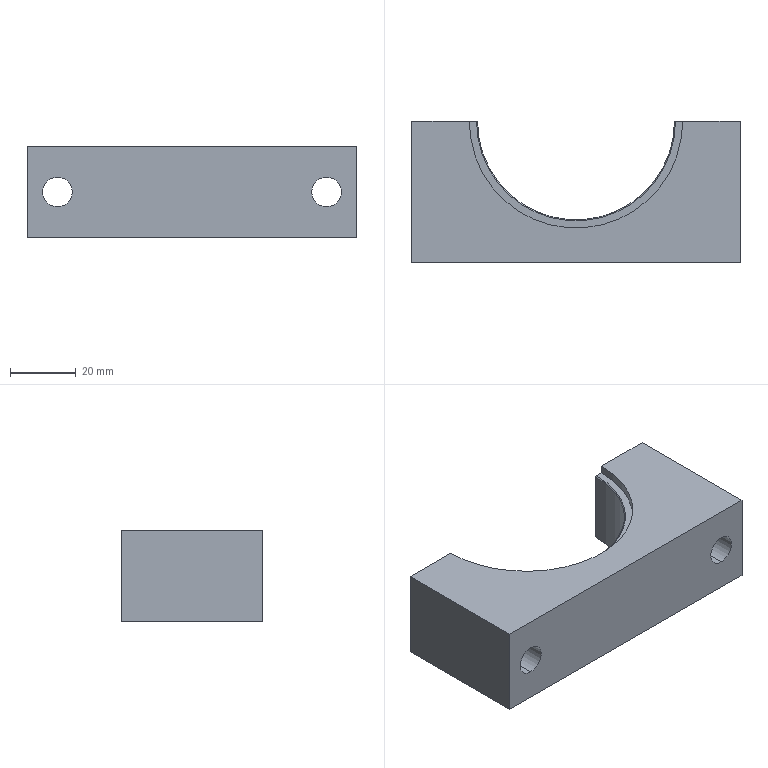Part | SolidWorks | features HoleWzd 2, ICE 2, Chamfer 1, Extrusion 1 | 1 solid | 21 faces | box 100 x 43 x 28 mm | volume 74059 mm3 | plane 10 | cylinder 9 | cone 2 | commonest cylinder face diameters 9 x4 4 x2 65 x2 60 x1
STEP:
#1=CARTESIAN_POINT('',(0.,-34.,12.));
#2=VERTEX_POINT('',#1);
#3=CARTESIAN_POINT('',(0.,-34.,16.));
#4=VERTEX_POINT('',#3);
#5=CARTESIAN_POINT('',(0.,-34.,14.));
#6=DIRECTION('',(0.,1.,0.));
#7=DIRECTION('',(0.,0.,1.));
#8=AXIS2_PLACEMENT_3D('',#5,#6,#7);
#9=CIRCLE('',#8,2.);
#10=EDGE_CURVE('',#2,#4,#9,.T.);
#11=ORIENTED_EDGE('',*,*,#10,.F.);
#12=CARTESIAN_POINT('',(0.,-30.,12.));
#13=VERTEX_POINT('',#12);
#14=CARTESIAN_POINT('',(0.,0.,12.));
#15=DIRECTION('',(0.,1.,0.));
#16=VECTOR('',#15,1000.);
#17=LINE('',#14,#16);
#18=EDGE_CURVE('',#2,#13,#17,.T.);
#19=ORIENTED_EDGE('',*,*,#18,.T.);
#20=CARTESIAN_POINT('',(0.,-30.,16.));
#21=VERTEX_POINT('',#20);
#22=CARTESIAN_POINT('',(0.,-30.,16.));
#23=CARTESIAN_POINT('',(-0.1322,-30.,16.));
#24=CARTESIAN_POINT('',(-0.2622,-29.999,15.987));
#25=CARTESIAN_POINT('',(-0.5178,-29.996,15.936));
#26=CARTESIAN_POINT('',(-0.6449,-29.993,15.898));
#27=CARTESIAN_POINT('',(-0.8871,-29.987,15.797));
#28=CARTESIAN_POINT('',(-1.002,-29.983,15.736));
#29=CARTESIAN_POINT('',(-1.219,-29.975,15.591));
#30=CARTESIAN_POINT('',(-1.322,-29.971,15.506));
#31=CARTESIAN_POINT('',(-1.599,-29.958,15.229));
#32=CARTESIAN_POINT('',(-1.748,-29.949,15.006));
#33=CARTESIAN_POINT('',(-1.947,-29.937,14.525));
#34=CARTESIAN_POINT('',(-2.,-29.933,14.262));
#35=CARTESIAN_POINT('',(-2.,-29.933,13.87));
#36=CARTESIAN_POINT('',(-1.987,-29.934,13.738));
#37=CARTESIAN_POINT('',(-1.936,-29.937,13.481));
#38=CARTESIAN_POINT('',(-1.898,-29.94,13.356));
#39=CARTESIAN_POINT('',(-1.798,-29.946,13.114));
#40=CARTESIAN_POINT('',(-1.735,-29.95,12.997));
#41=CARTESIAN_POINT('',(-1.591,-29.958,12.78));
#42=CARTESIAN_POINT('',(-1.508,-29.962,12.679));
#43=CARTESIAN_POINT('',(-1.321,-29.971,12.493));
#44=CARTESIAN_POINT('',(-1.22,-29.975,12.41));
#45=CARTESIAN_POINT('',(-1.003,-29.983,12.265));
#46=CARTESIAN_POINT('',(-0.8865,-29.987,12.202));
#47=CARTESIAN_POINT('',(-0.6442,-29.993,12.102));
#48=CARTESIAN_POINT('',(-0.5195,-29.996,12.064));
#49=CARTESIAN_POINT('',(-0.2631,-29.999,12.013));
#50=CARTESIAN_POINT('',(-0.1305,-30.,12.));
#51=CARTESIAN_POINT('',(0.,-30.,12.));
#52=B_SPLINE_CURVE_WITH_KNOTS('',3,(#22,#23,#24,#25,#26,#27,#28,#29,#30,#31,#32,#33,#34,#35,#36,#37,#38,#39,#40,#41,#42,#43,#44,#45,#46,#47,#48,#49,#50,#51),.UNSPECIFIED.,.F.,.F.,(4,2,2,2,2,2,2,2,2,2,2,2,2,2,4),(0.,0.0003909,0.0007818,0.001173,0.001564,0.002345,0.003127,0.003518,0.003909,0.0043,0.004691,0.005082,0.005473,0.005864,0.006255),.UNSPECIFIED.);
#53=EDGE_CURVE('',#21,#13,#52,.T.);
#54=ORIENTED_EDGE('',*,*,#53,.F.);
#55=CARTESIAN_POINT('',(0.,0.,16.));
#56=DIRECTION('',(0.,1.,0.));
#57=VECTOR('',#56,1000.);
#58=LINE('',#55,#57);
#59=EDGE_CURVE('',#4,#21,#58,.T.);
#60=ORIENTED_EDGE('',*,*,#59,.F.);
#61=EDGE_LOOP('',(#11,#19,#54,#60));
#62=FACE_OUTER_BOUND('',#61,.T.);
#63=CARTESIAN_POINT('',(0.,0.,14.));
#64=DIRECTION('',(0.,1.,0.));
#65=DIRECTION('',(0.,0.,1.));
#66=AXIS2_PLACEMENT_3D('',#63,#64,#65);
#67=CYLINDRICAL_SURFACE('',#66,2.);
#68=ADVANCED_FACE('',(#62),#67,.F.);
#69=CARTESIAN_POINT('',(-41.,-43.,9.5));
#70=VERTEX_POINT('',#69);
#71=CARTESIAN_POINT('',(-41.,-43.,18.5));
#72=VERTEX_POINT('',#71);
#73=CARTESIAN_POINT('',(-41.,-43.,14.));
#74=DIRECTION('',(0.,1.,0.));
#75=DIRECTION('',(0.,0.,1.));
#76=AXIS2_PLACEMENT_3D('',#73,#74,#75);
#77=CIRCLE('',#76,4.5);
#78=EDGE_CURVE('',#70,#72,#77,.T.);
#79=ORIENTED_EDGE('',*,*,#78,.F.);
#80=CARTESIAN_POINT('',(-41.,0.,9.5));
#81=VERTEX_POINT('',#80);
#82=CARTESIAN_POINT('',(-41.,0.,9.5));
#83=DIRECTION('',(0.,1.,0.));
#84=VECTOR('',#83,1000.);
#85=LINE('',#82,#84);
#86=EDGE_CURVE('',#70,#81,#85,.T.);
#87=ORIENTED_EDGE('',*,*,#86,.T.);
#88=CARTESIAN_POINT('',(-41.,0.,18.5));
#89=VERTEX_POINT('',#88);
#90=CARTESIAN_POINT('',(-41.,0.,14.));
#91=DIRECTION('',(0.,1.,0.));
#92=DIRECTION('',(0.,0.,1.));
#93=AXIS2_PLACEMENT_3D('',#90,#91,#92);
#94=CIRCLE('',#93,4.5);
#95=EDGE_CURVE('',#81,#89,#94,.T.);
#96=ORIENTED_EDGE('',*,*,#95,.T.);
#97=CARTESIAN_POINT('',(-41.,0.,18.5));
#98=DIRECTION('',(0.,1.,0.));
#99=VECTOR('',#98,1000.);
#100=LINE('',#97,#99);
#101=EDGE_CURVE('',#72,#89,#100,.T.);
#102=ORIENTED_EDGE('',*,*,#101,.F.);
#103=EDGE_LOOP('',(#79,#87,#96,#102));
#104=FACE_OUTER_BOUND('',#103,.T.);
#105=CARTESIAN_POINT('',(-41.,0.,14.));
#106=DIRECTION('',(0.,1.,0.));
#107=DIRECTION('',(0.,0.,1.));
#108=AXIS2_PLACEMENT_3D('',#105,#106,#107);
#109=CYLINDRICAL_SURFACE('',#108,4.5);
#110=ADVANCED_FACE('',(#104),#109,.F.);
#111=CARTESIAN_POINT('',(41.,-43.,9.5));
#112=VERTEX_POINT('',#111);
#113=CARTESIAN_POINT('',(41.,-43.,18.5));
#114=VERTEX_POINT('',#113);
#115=CARTESIAN_POINT('',(41.,-43.,14.));
#116=DIRECTION('',(0.,1.,0.));
#117=DIRECTION('',(0.,0.,1.));
#118=AXIS2_PLACEMENT_3D('',#115,#116,#117);
#119=CIRCLE('',#118,4.5);
#120=EDGE_CURVE('',#112,#114,#119,.T.);
#121=ORIENTED_EDGE('',*,*,#120,.F.);
#122=CARTESIAN_POINT('',(41.,0.,9.5));
#123=VERTEX_POINT('',#122);
#124=CARTESIAN_POINT('',(41.,0.,9.5));
#125=DIRECTION('',(0.,1.,0.));
#126=VECTOR('',#125,1000.);
#127=LINE('',#124,#126);
#128=EDGE_CURVE('',#112,#123,#127,.T.);
#129=ORIENTED_EDGE('',*,*,#128,.T.);
#130=CARTESIAN_POINT('',(41.,0.,18.5));
#131=VERTEX_POINT('',#130);
#132=CARTESIAN_POINT('',(41.,0.,14.));
#133=DIRECTION('',(0.,1.,0.));
#134=DIRECTION('',(0.,0.,1.));
#135=AXIS2_PLACEMENT_3D('',#132,#133,#134);
#136=CIRCLE('',#135,4.5);
#137=EDGE_CURVE('',#123,#131,#136,.T.);
#138=ORIENTED_EDGE('',*,*,#137,.T.);
#139=CARTESIAN_POINT('',(41.,0.,18.5));
#140=DIRECTION('',(0.,1.,0.));
#141=VECTOR('',#140,1000.);
#142=LINE('',#139,#141);
#143=EDGE_CURVE('',#114,#131,#142,.T.);
#144=ORIENTED_EDGE('',*,*,#143,.F.);
#145=EDGE_LOOP('',(#121,#129,#138,#144));
#146=FACE_OUTER_BOUND('',#145,.T.);
#147=CARTESIAN_POINT('',(41.,0.,14.));
#148=DIRECTION('',(0.,1.,0.));
#149=DIRECTION('',(0.,0.,1.));
#150=AXIS2_PLACEMENT_3D('',#147,#148,#149);
#151=CYLINDRICAL_SURFACE('',#150,4.5);
#152=ADVANCED_FACE('',(#146),#151,.F.);
#153=ORIENTED_EDGE('',*,*,#53,.T.);
#154=CARTESIAN_POINT('',(0.,-30.,12.));
#155=CARTESIAN_POINT('',(0.261,-30.,12.));
#156=CARTESIAN_POINT('',(0.5242,-29.996,12.052));
#157=CARTESIAN_POINT('',(1.006,-29.984,12.252));
#158=CARTESIAN_POINT('',(1.229,-29.975,12.401));
#159=CARTESIAN_POINT('',(1.505,-29.962,12.677));
#160=CARTESIAN_POINT('',(1.59,-29.958,12.78));
#161=CARTESIAN_POINT('',(1.735,-29.95,12.997));
#162=CARTESIAN_POINT('',(1.797,-29.946,13.112));
#163=CARTESIAN_POINT('',(1.897,-29.94,13.354));
#164=CARTESIAN_POINT('',(1.936,-29.937,13.481));
#165=CARTESIAN_POINT('',(1.987,-29.934,13.737));
#166=CARTESIAN_POINT('',(2.,-29.933,13.866));
#167=CARTESIAN_POINT('',(2.,-29.933,14.13));
#168=CARTESIAN_POINT('',(1.987,-29.934,14.261));
#169=CARTESIAN_POINT('',(1.937,-29.937,14.516));
#170=CARTESIAN_POINT('',(1.898,-29.94,14.643));
#171=CARTESIAN_POINT('',(1.798,-29.946,14.886));
#172=CARTESIAN_POINT('',(1.737,-29.95,15.001));
#173=CARTESIAN_POINT('',(1.592,-29.958,15.218));
#174=CARTESIAN_POINT('',(1.507,-29.962,15.321));
#175=CARTESIAN_POINT('',(1.323,-29.971,15.506));
#176=CARTESIAN_POINT('',(1.222,-29.975,15.588));
#177=CARTESIAN_POINT('',(1.004,-29.983,15.735));
#178=CARTESIAN_POINT('',(0.8877,-29.987,15.797));
#179=CARTESIAN_POINT('',(0.5269,-29.996,15.947));
#180=CARTESIAN_POINT('',(0.2643,-30.,16.));
#181=CARTESIAN_POINT('',(0.,-30.,16.));
#182=B_SPLINE_CURVE_WITH_KNOTS('',3,(#154,#155,#156,#157,#158,#159,#160,#161,#162,#163,#164,#165,#166,#167,#168,#169,#170,#171,#172,#173,#174,#175,#176,#177,#178,#179,#180,#181),.UNSPECIFIED.,.F.,.F.,(4,2,2,2,2,2,2,2,2,2,2,2,2,4),(0.006255,0.007036,0.007818,0.008209,0.0086,0.00899,0.009381,0.009772,0.01016,0.01055,0.01094,0.01134,0.01173,0.01251),.UNSPECIFIED.);
#183=EDGE_CURVE('',#13,#21,#182,.T.);
#184=ORIENTED_EDGE('',*,*,#183,.T.);
#185=EDGE_LOOP('',(#153,#184));
#186=FACE_BOUND('',#185,.T.);
#187=CARTESIAN_POINT('',(30.,0.,25.2));
#188=VERTEX_POINT('',#187);
#189=CARTESIAN_POINT('',(30.,0.,2.8));
#190=VERTEX_POINT('',#189);
#191=CARTESIAN_POINT('',(30.,0.,28.));
#192=DIRECTION('',(0.,0.,-1.));
#193=VECTOR('',#192,1000.);
#194=LINE('',#191,#193);
#195=EDGE_CURVE('',#188,#190,#194,.T.);
#196=ORIENTED_EDGE('',*,*,#195,.T.);
#197=CARTESIAN_POINT('',(-30.,0.,2.8));
#198=VERTEX_POINT('',#197);
#199=CARTESIAN_POINT('',(0.,0.,2.8));
#200=DIRECTION('',(0.,0.,-1.));
#201=DIRECTION('',(-1.,0.,0.));
#202=AXIS2_PLACEMENT_3D('',#199,#200,#201);
#203=CIRCLE('',#202,30.);
#204=EDGE_CURVE('',#190,#198,#203,.T.);
#205=ORIENTED_EDGE('',*,*,#204,.T.);
#206=CARTESIAN_POINT('',(-30.,0.,25.2));
#207=VERTEX_POINT('',#206);
#208=CARTESIAN_POINT('',(-30.,0.,28.));
#209=DIRECTION('',(0.,0.,-1.));
#210=VECTOR('',#209,1000.);
#211=LINE('',#208,#210);
#212=EDGE_CURVE('',#207,#198,#211,.T.);
#213=ORIENTED_EDGE('',*,*,#212,.F.);
#214=CARTESIAN_POINT('',(0.,0.,25.2));
#215=DIRECTION('',(0.,0.,1.));
#216=DIRECTION('',(1.,0.,0.));
#217=AXIS2_PLACEMENT_3D('',#214,#215,#216);
#218=CIRCLE('',#217,30.);
#219=EDGE_CURVE('',#207,#188,#218,.T.);
#220=ORIENTED_EDGE('',*,*,#219,.T.);
#221=EDGE_LOOP('',(#196,#205,#213,#220));
#222=FACE_OUTER_BOUND('',#221,.T.);
#223=CARTESIAN_POINT('',(0.,0.,28.));
#224=DIRECTION('',(0.,0.,-1.));
#225=DIRECTION('',(-1.,0.,0.));
#226=AXIS2_PLACEMENT_3D('',#223,#224,#225);
#227=CYLINDRICAL_SURFACE('',#226,30.);
#228=ADVANCED_FACE('',(#186,#222),#227,.F.);
#229=CARTESIAN_POINT('',(-41.,0.,14.));
#230=DIRECTION('',(0.,1.,0.));
#231=DIRECTION('',(0.,0.,1.));
#232=AXIS2_PLACEMENT_3D('',#229,#230,#231);
#233=CIRCLE('',#232,4.5);
#234=EDGE_CURVE('',#89,#81,#233,.T.);
#235=ORIENTED_EDGE('',*,*,#234,.F.);
#236=ORIENTED_EDGE('',*,*,#95,.F.);
#237=EDGE_LOOP('',(#235,#236));
#238=FACE_BOUND('',#237,.T.);
#239=ORIENTED_EDGE('',*,*,#212,.T.);
#240=CARTESIAN_POINT('',(-30.3,0.,2.5));
#241=VERTEX_POINT('',#240);
#242=CARTESIAN_POINT('',(0.,0.,32.8));
#243=DIRECTION('',(-0.7071,0.,-0.7071));
#244=VECTOR('',#243,1000.);
#245=LINE('',#242,#244);
#246=EDGE_CURVE('',#198,#241,#245,.T.);
#247=ORIENTED_EDGE('',*,*,#246,.T.);
#248=CARTESIAN_POINT('',(-32.5,0.,2.5));
#249=VERTEX_POINT('',#248);
#250=CARTESIAN_POINT('',(-50.,0.,2.5));
#251=DIRECTION('',(1.,0.,0.));
#252=VECTOR('',#251,1000.);
#253=LINE('',#250,#252);
#254=EDGE_CURVE('',#249,#241,#253,.T.);
#255=ORIENTED_EDGE('',*,*,#254,.F.);
#256=CARTESIAN_POINT('',(-32.5,0.,0.));
#257=VERTEX_POINT('',#256);
#258=CARTESIAN_POINT('',(-32.5,0.,2.5));
#259=DIRECTION('',(0.,0.,-1.));
#260=VECTOR('',#259,1000.);
#261=LINE('',#258,#260);
#262=EDGE_CURVE('',#249,#257,#261,.T.);
#263=ORIENTED_EDGE('',*,*,#262,.T.);
#264=CARTESIAN_POINT('',(-50.,0.,0.));
#265=VERTEX_POINT('',#264);
#266=CARTESIAN_POINT('',(-50.,0.,0.));
#267=DIRECTION('',(-1.,0.,0.));
#268=VECTOR('',#267,1000.);
#269=LINE('',#266,#268);
#270=EDGE_CURVE('',#257,#265,#269,.T.);
#271=ORIENTED_EDGE('',*,*,#270,.T.);
#272=CARTESIAN_POINT('',(-50.,0.,28.));
#273=VERTEX_POINT('',#272);
#274=CARTESIAN_POINT('',(-50.,0.,28.));
#275=DIRECTION('',(0.,0.,-1.));
#276=VECTOR('',#275,1000.);
#277=LINE('',#274,#276);
#278=EDGE_CURVE('',#273,#265,#277,.T.);
#279=ORIENTED_EDGE('',*,*,#278,.F.);
#280=CARTESIAN_POINT('',(-32.5,0.,28.));
#281=VERTEX_POINT('',#280);
#282=CARTESIAN_POINT('',(-50.,0.,28.));
#283=DIRECTION('',(-1.,0.,0.));
#284=VECTOR('',#283,1000.);
#285=LINE('',#282,#284);
#286=EDGE_CURVE('',#281,#273,#285,.T.);
#287=ORIENTED_EDGE('',*,*,#286,.F.);
#288=CARTESIAN_POINT('',(-32.5,0.,25.5));
#289=VERTEX_POINT('',#288);
#290=CARTESIAN_POINT('',(-32.5,0.,25.5));
#291=DIRECTION('',(0.,0.,-1.));
#292=VECTOR('',#291,1000.);
#293=LINE('',#290,#292);
#294=EDGE_CURVE('',#281,#289,#293,.T.);
#295=ORIENTED_EDGE('',*,*,#294,.T.);
#296=CARTESIAN_POINT('',(-30.3,0.,25.5));
#297=VERTEX_POINT('',#296);
#298=CARTESIAN_POINT('',(-50.,0.,25.5));
#299=DIRECTION('',(-1.,0.,0.));
#300=VECTOR('',#299,1000.);
#301=LINE('',#298,#300);
#302=EDGE_CURVE('',#297,#289,#301,.T.);
#303=ORIENTED_EDGE('',*,*,#302,.F.);
#304=CARTESIAN_POINT('',(0.,0.,-4.8));
#305=DIRECTION('',(0.7071,0.,-0.7071));
#306=VECTOR('',#305,1000.);
#307=LINE('',#304,#306);
#308=EDGE_CURVE('',#297,#207,#307,.T.);
#309=ORIENTED_EDGE('',*,*,#308,.T.);
#310=EDGE_LOOP('',(#239,#247,#255,#263,#271,#279,#287,#295,#303,#309));
#311=FACE_OUTER_BOUND('',#310,.T.);
#312=CARTESIAN_POINT('',(-50.,0.,28.));
#313=DIRECTION('',(0.,-1.,0.));
#314=DIRECTION('',(1.,0.,0.));
#315=AXIS2_PLACEMENT_3D('',#312,#313,#314);
#316=PLANE('',#315);
#317=ADVANCED_FACE('',(#238,#311),#316,.F.);
#318=CARTESIAN_POINT('',(-50.,-43.,0.));
#319=VERTEX_POINT('',#318);
#320=CARTESIAN_POINT('',(-50.,-43.,0.));
#321=DIRECTION('',(0.,-1.,0.));
#322=VECTOR('',#321,1000.);
#323=LINE('',#320,#322);
#324=EDGE_CURVE('',#265,#319,#323,.T.);
#325=ORIENTED_EDGE('',*,*,#324,.T.);
#326=CARTESIAN_POINT('',(-50.,-43.,28.));
#327=VERTEX_POINT('',#326);
#328=CARTESIAN_POINT('',(-50.,-43.,28.));
#329=DIRECTION('',(0.,0.,-1.));
#330=VECTOR('',#329,1000.);
#331=LINE('',#328,#330);
#332=EDGE_CURVE('',#327,#319,#331,.T.);
#333=ORIENTED_EDGE('',*,*,#332,.F.);
#334=CARTESIAN_POINT('',(-50.,-43.,28.));
#335=DIRECTION('',(0.,-1.,0.));
#336=VECTOR('',#335,1000.);
#337=LINE('',#334,#336);
#338=EDGE_CURVE('',#273,#327,#337,.T.);
#339=ORIENTED_EDGE('',*,*,#338,.F.);
#340=ORIENTED_EDGE('',*,*,#278,.T.);
#341=EDGE_LOOP('',(#325,#333,#339,#340));
#342=FACE_OUTER_BOUND('',#341,.T.);
#343=CARTESIAN_POINT('',(-50.,-43.,28.));
#344=DIRECTION('',(1.,0.,0.));
#345=DIRECTION('',(0.,0.,-1.));
#346=AXIS2_PLACEMENT_3D('',#343,#344,#345);
#347=PLANE('',#346);
#348=ADVANCED_FACE('',(#342),#347,.F.);
#349=CARTESIAN_POINT('',(-41.,-43.,14.));
#350=DIRECTION('',(0.,1.,0.));
#351=DIRECTION('',(0.,0.,1.));
#352=AXIS2_PLACEMENT_3D('',#349,#350,#351);
#353=CIRCLE('',#352,4.5);
#354=EDGE_CURVE('',#72,#70,#353,.T.);
#355=ORIENTED_EDGE('',*,*,#354,.T.);
#356=ORIENTED_EDGE('',*,*,#78,.T.);
#357=EDGE_LOOP('',(#355,#356));
#358=FACE_BOUND('',#357,.T.);
#359=CARTESIAN_POINT('',(41.,-43.,14.));
#360=DIRECTION('',(0.,1.,0.));
#361=DIRECTION('',(0.,0.,1.));
#362=AXIS2_PLACEMENT_3D('',#359,#360,#361);
#363=CIRCLE('',#362,4.5);
#364=EDGE_CURVE('',#114,#112,#363,.T.);
#365=ORIENTED_EDGE('',*,*,#364,.T.);
#366=ORIENTED_EDGE('',*,*,#120,.T.);
#367=EDGE_LOOP('',(#365,#366));
#368=FACE_BOUND('',#367,.T.);
#369=CARTESIAN_POINT('',(50.,-43.,0.));
#370=VERTEX_POINT('',#369);
#371=CARTESIAN_POINT('',(-50.,-43.,0.));
#372=DIRECTION('',(1.,0.,0.));
#373=VECTOR('',#372,1000.);
#374=LINE('',#371,#373);
#375=EDGE_CURVE('',#319,#370,#374,.T.);
#376=ORIENTED_EDGE('',*,*,#375,.T.);
#377=CARTESIAN_POINT('',(50.,-43.,28.));
#378=VERTEX_POINT('',#377);
#379=CARTESIAN_POINT('',(50.,-43.,28.));
#380=DIRECTION('',(0.,0.,-1.));
#381=VECTOR('',#380,1000.);
#382=LINE('',#379,#381);
#383=EDGE_CURVE('',#378,#370,#382,.T.);
#384=ORIENTED_EDGE('',*,*,#383,.F.);
#385=CARTESIAN_POINT('',(-50.,-43.,28.));
#386=DIRECTION('',(1.,0.,0.));
#387=VECTOR('',#386,1000.);
#388=LINE('',#385,#387);
#389=EDGE_CURVE('',#327,#378,#388,.T.);
#390=ORIENTED_EDGE('',*,*,#389,.F.);
#391=ORIENTED_EDGE('',*,*,#332,.T.);
#392=EDGE_LOOP('',(#376,#384,#390,#391));
#393=FACE_OUTER_BOUND('',#392,.T.);
#394=CARTESIAN_POINT('',(-50.,-43.,28.));
#395=DIRECTION('',(0.,1.,0.));
#396=DIRECTION('',(-1.,0.,0.));
#397=AXIS2_PLACEMENT_3D('',#394,#395,#396);
#398=PLANE('',#397);
#399=ADVANCED_FACE('',(#358,#368,#393),#398,.F.);
#400=CARTESIAN_POINT('',(50.,0.,0.));
#401=VERTEX_POINT('',#400);
#402=CARTESIAN_POINT('',(50.,-43.,0.));
#403=DIRECTION('',(0.,1.,0.));
#404=VECTOR('',#403,1000.);
#405=LINE('',#402,#404);
#406=EDGE_CURVE('',#370,#401,#405,.T.);
#407=ORIENTED_EDGE('',*,*,#406,.T.);
#408=CARTESIAN_POINT('',(50.,0.,28.));
#409=VERTEX_POINT('',#408);
#410=CARTESIAN_POINT('',(50.,0.,28.));
#411=DIRECTION('',(0.,0.,-1.));
#412=VECTOR('',#411,1000.);
#413=LINE('',#410,#412);
#414=EDGE_CURVE('',#409,#401,#413,.T.);
#415=ORIENTED_EDGE('',*,*,#414,.F.);
#416=CARTESIAN_POINT('',(50.,-43.,28.));
#417=DIRECTION('',(0.,1.,0.));
#418=VECTOR('',#417,1000.);
#419=LINE('',#416,#418);
#420=EDGE_CURVE('',#378,#409,#419,.T.);
#421=ORIENTED_EDGE('',*,*,#420,.F.);
#422=ORIENTED_EDGE('',*,*,#383,.T.);
#423=EDGE_LOOP('',(#407,#415,#421,#422));
#424=FACE_OUTER_BOUND('',#423,.T.);
#425=CARTESIAN_POINT('',(50.,-43.,28.));
#426=DIRECTION('',(-1.,0.,0.));
#427=DIRECTION('',(0.,-1.,0.));
#428=AXIS2_PLACEMENT_3D('',#425,#426,#427);
#429=PLANE('',#428);
#430=ADVANCED_FACE('',(#424),#429,.F.);
#431=CARTESIAN_POINT('',(41.,0.,14.));
#432=DIRECTION('',(0.,1.,0.));
#433=DIRECTION('',(0.,0.,1.));
#434=AXIS2_PLACEMENT_3D('',#431,#432,#433);
#435=CIRCLE('',#434,4.5);
#436=EDGE_CURVE('',#131,#123,#435,.T.);
#437=ORIENTED_EDGE('',*,*,#436,.F.);
#438=ORIENTED_EDGE('',*,*,#137,.F.);
#439=EDGE_LOOP('',(#437,#438));
#440=FACE_BOUND('',#439,.T.);
#441=CARTESIAN_POINT('',(30.3,0.,2.5));
#442=VERTEX_POINT('',#441);
#443=CARTESIAN_POINT('',(32.5,0.,2.5));
#444=VERTEX_POINT('',#443);
#445=CARTESIAN_POINT('',(30.,0.,2.5));
#446=DIRECTION('',(1.,0.,0.));
#447=VECTOR('',#446,1000.);
#448=LINE('',#445,#447);
#449=EDGE_CURVE('',#442,#444,#448,.T.);
#450=ORIENTED_EDGE('',*,*,#449,.F.);
#451=CARTESIAN_POINT('',(0.,0.,32.8));
#452=DIRECTION('',(-0.7071,0.,0.7071));
#453=VECTOR('',#452,1000.);
#454=LINE('',#451,#453);
#455=EDGE_CURVE('',#442,#190,#454,.T.);
#456=ORIENTED_EDGE('',*,*,#455,.T.);
#457=ORIENTED_EDGE('',*,*,#195,.F.);
#458=CARTESIAN_POINT('',(30.3,0.,25.5));
#459=VERTEX_POINT('',#458);
#460=CARTESIAN_POINT('',(0.,0.,-4.8));
#461=DIRECTION('',(0.7071,0.,0.7071));
#462=VECTOR('',#461,1000.);
#463=LINE('',#460,#462);
#464=EDGE_CURVE('',#188,#459,#463,.T.);
#465=ORIENTED_EDGE('',*,*,#464,.T.);
#466=CARTESIAN_POINT('',(32.5,0.,25.5));
#467=VERTEX_POINT('',#466);
#468=CARTESIAN_POINT('',(30.,0.,25.5));
#469=DIRECTION('',(-1.,0.,0.));
#470=VECTOR('',#469,1000.);
#471=LINE('',#468,#470);
#472=EDGE_CURVE('',#467,#459,#471,.T.);
#473=ORIENTED_EDGE('',*,*,#472,.F.);
#474=CARTESIAN_POINT('',(32.5,0.,28.));
#475=VERTEX_POINT('',#474);
#476=CARTESIAN_POINT('',(32.5,0.,25.5));
#477=DIRECTION('',(0.,0.,1.));
#478=VECTOR('',#477,1000.);
#479=LINE('',#476,#478);
#480=EDGE_CURVE('',#467,#475,#479,.T.);
#481=ORIENTED_EDGE('',*,*,#480,.T.);
#482=CARTESIAN_POINT('',(30.,0.,28.));
#483=DIRECTION('',(-1.,0.,0.));
#484=VECTOR('',#483,1000.);
#485=LINE('',#482,#484);
#486=EDGE_CURVE('',#409,#475,#485,.T.);
#487=ORIENTED_EDGE('',*,*,#486,.F.);
#488=ORIENTED_EDGE('',*,*,#414,.T.);
#489=CARTESIAN_POINT('',(32.5,0.,0.));
#490=VERTEX_POINT('',#489);
#491=CARTESIAN_POINT('',(30.,0.,0.));
#492=DIRECTION('',(-1.,0.,0.));
#493=VECTOR('',#492,1000.);
#494=LINE('',#491,#493);
#495=EDGE_CURVE('',#401,#490,#494,.T.);
#496=ORIENTED_EDGE('',*,*,#495,.T.);
#497=CARTESIAN_POINT('',(32.5,0.,2.5));
#498=DIRECTION('',(0.,0.,1.));
#499=VECTOR('',#498,1000.);
#500=LINE('',#497,#499);
#501=EDGE_CURVE('',#490,#444,#500,.T.);
#502=ORIENTED_EDGE('',*,*,#501,.T.);
#503=EDGE_LOOP('',(#450,#456,#457,#465,#473,#481,#487,#488,#496,#502));
#504=FACE_OUTER_BOUND('',#503,.T.);
#505=CARTESIAN_POINT('',(30.,0.,28.));
#506=DIRECTION('',(0.,-1.,0.));
#507=DIRECTION('',(1.,0.,0.));
#508=AXIS2_PLACEMENT_3D('',#505,#506,#507);
#509=PLANE('',#508);
#510=ADVANCED_FACE('',(#440,#504),#509,.F.);
#511=CARTESIAN_POINT('',(0.,0.,28.));
#512=DIRECTION('',(0.,0.,1.));
#513=DIRECTION('',(1.,0.,0.));
#514=AXIS2_PLACEMENT_3D('',#511,#512,#513);
#515=CIRCLE('',#514,32.5);
#516=EDGE_CURVE('',#281,#475,#515,.T.);
#517=ORIENTED_EDGE('',*,*,#516,.F.);
#518=ORIENTED_EDGE('',*,*,#286,.T.);
#519=ORIENTED_EDGE('',*,*,#338,.T.);
#520=ORIENTED_EDGE('',*,*,#389,.T.);
#521=ORIENTED_EDGE('',*,*,#420,.T.);
#522=ORIENTED_EDGE('',*,*,#486,.T.);
#523=EDGE_LOOP('',(#517,#518,#519,#520,#521,#522));
#524=FACE_OUTER_BOUND('',#523,.T.);
#525=CARTESIAN_POINT('',(0.,0.,28.));
#526=DIRECTION('',(0.,0.,1.));
#527=DIRECTION('',(1.,0.,0.));
#528=AXIS2_PLACEMENT_3D('',#525,#526,#527);
#529=PLANE('',#528);
#530=ADVANCED_FACE('',(#524),#529,.T.);
#531=ORIENTED_EDGE('',*,*,#270,.F.);
#532=CARTESIAN_POINT('',(0.,0.,0.));
#533=DIRECTION('',(0.,0.,1.));
#534=DIRECTION('',(1.,0.,0.));
#535=AXIS2_PLACEMENT_3D('',#532,#533,#534);
#536=CIRCLE('',#535,32.5);
#537=EDGE_CURVE('',#257,#490,#536,.T.);
#538=ORIENTED_EDGE('',*,*,#537,.T.);
#539=ORIENTED_EDGE('',*,*,#495,.F.);
#540=ORIENTED_EDGE('',*,*,#406,.F.);
#541=ORIENTED_EDGE('',*,*,#375,.F.);
#542=ORIENTED_EDGE('',*,*,#324,.F.);
#543=EDGE_LOOP('',(#531,#538,#539,#540,#541,#542));
#544=FACE_OUTER_BOUND('',#543,.T.);
#545=CARTESIAN_POINT('',(0.,0.,0.));
#546=DIRECTION('',(0.,0.,1.));
#547=DIRECTION('',(1.,0.,0.));
#548=AXIS2_PLACEMENT_3D('',#545,#546,#547);
#549=PLANE('',#548);
#550=ADVANCED_FACE('',(#544),#549,.F.);
#551=ORIENTED_EDGE('',*,*,#472,.T.);
#552=CARTESIAN_POINT('',(0.,0.,25.5));
#553=DIRECTION('',(0.,0.,-1.));
#554=DIRECTION('',(1.,0.,0.));
#555=AXIS2_PLACEMENT_3D('',#552,#553,#554);
#556=CIRCLE('',#555,30.3);
#557=EDGE_CURVE('',#459,#297,#556,.T.);
#558=ORIENTED_EDGE('',*,*,#557,.T.);
#559=ORIENTED_EDGE('',*,*,#302,.T.);
#560=CARTESIAN_POINT('',(0.,0.,25.5));
#561=DIRECTION('',(0.,0.,1.));
#562=DIRECTION('',(1.,0.,0.));
#563=AXIS2_PLACEMENT_3D('',#560,#561,#562);
#564=CIRCLE('',#563,32.5);
#565=EDGE_CURVE('',#289,#467,#564,.T.);
#566=ORIENTED_EDGE('',*,*,#565,.T.);
#567=EDGE_LOOP('',(#551,#558,#559,#566));
#568=FACE_OUTER_BOUND('',#567,.T.);
#569=CARTESIAN_POINT('',(0.,0.,25.5));
#570=DIRECTION('',(0.,0.,1.));
#571=DIRECTION('',(1.,0.,0.));
#572=AXIS2_PLACEMENT_3D('',#569,#570,#571);
#573=PLANE('',#572);
#574=ADVANCED_FACE('',(#568),#573,.T.);
#575=ORIENTED_EDGE('',*,*,#516,.T.);
#576=ORIENTED_EDGE('',*,*,#480,.F.);
#577=ORIENTED_EDGE('',*,*,#565,.F.);
#578=ORIENTED_EDGE('',*,*,#294,.F.);
#579=EDGE_LOOP('',(#575,#576,#577,#578));
#580=FACE_OUTER_BOUND('',#579,.T.);
#581=CARTESIAN_POINT('',(0.,0.,25.5));
#582=DIRECTION('',(0.,0.,1.));
#583=DIRECTION('',(1.,0.,0.));
#584=AXIS2_PLACEMENT_3D('',#581,#582,#583);
#585=CYLINDRICAL_SURFACE('',#584,32.5);
#586=ADVANCED_FACE('',(#580),#585,.F.);
#587=ORIENTED_EDGE('',*,*,#254,.T.);
#588=CARTESIAN_POINT('',(0.,0.,2.5));
#589=DIRECTION('',(0.,0.,1.));
#590=DIRECTION('',(-1.,0.,0.));
#591=AXIS2_PLACEMENT_3D('',#588,#589,#590);
#592=CIRCLE('',#591,30.3);
#593=EDGE_CURVE('',#241,#442,#592,.T.);
#594=ORIENTED_EDGE('',*,*,#593,.T.);
#595=ORIENTED_EDGE('',*,*,#449,.T.);
#596=CARTESIAN_POINT('',(0.,0.,2.5));
#597=DIRECTION('',(0.,0.,-1.));
#598=DIRECTION('',(-1.,0.,0.));
#599=AXIS2_PLACEMENT_3D('',#596,#597,#598);
#600=CIRCLE('',#599,32.5);
#601=EDGE_CURVE('',#444,#249,#600,.T.);
#602=ORIENTED_EDGE('',*,*,#601,.T.);
#603=EDGE_LOOP('',(#587,#594,#595,#602));
#604=FACE_OUTER_BOUND('',#603,.T.);
#605=CARTESIAN_POINT('',(0.,0.,2.5));
#606=DIRECTION('',(0.,0.,-1.));
#607=DIRECTION('',(-1.,0.,0.));
#608=AXIS2_PLACEMENT_3D('',#605,#606,#607);
#609=PLANE('',#608);
#610=ADVANCED_FACE('',(#604),#609,.T.);
#611=ORIENTED_EDGE('',*,*,#601,.F.);
#612=ORIENTED_EDGE('',*,*,#501,.F.);
#613=ORIENTED_EDGE('',*,*,#537,.F.);
#614=ORIENTED_EDGE('',*,*,#262,.F.);
#615=EDGE_LOOP('',(#611,#612,#613,#614));
#616=FACE_OUTER_BOUND('',#615,.T.);
#617=CARTESIAN_POINT('',(0.,0.,2.5));
#618=DIRECTION('',(0.,0.,-1.));
#619=DIRECTION('',(-1.,0.,0.));
#620=AXIS2_PLACEMENT_3D('',#617,#618,#619);
#621=CYLINDRICAL_SURFACE('',#620,32.5);
#622=ADVANCED_FACE('',(#616),#621,.F.);
#623=ORIENTED_EDGE('',*,*,#246,.F.);
#624=ORIENTED_EDGE('',*,*,#204,.F.);
#625=ORIENTED_EDGE('',*,*,#455,.F.);
#626=ORIENTED_EDGE('',*,*,#593,.F.);
#627=EDGE_LOOP('',(#623,#624,#625,#626));
#628=FACE_OUTER_BOUND('',#627,.T.);
#629=CARTESIAN_POINT('',(0.,0.,2.5));
#630=DIRECTION('',(0.,0.,-1.));
#631=DIRECTION('',(-1.,0.,0.));
#632=AXIS2_PLACEMENT_3D('',#629,#630,#631);
#633=CONICAL_SURFACE('',#632,30.3,0.7854);
#634=ADVANCED_FACE('',(#628),#633,.F.);
#635=ORIENTED_EDGE('',*,*,#464,.F.);
#636=ORIENTED_EDGE('',*,*,#219,.F.);
#637=ORIENTED_EDGE('',*,*,#308,.F.);
#638=ORIENTED_EDGE('',*,*,#557,.F.);
#639=EDGE_LOOP('',(#635,#636,#637,#638));
#640=FACE_OUTER_BOUND('',#639,.T.);
#641=CARTESIAN_POINT('',(0.,0.,25.5));
#642=DIRECTION('',(0.,0.,1.));
#643=DIRECTION('',(1.,0.,0.));
#644=AXIS2_PLACEMENT_3D('',#641,#642,#643);
#645=CONICAL_SURFACE('',#644,30.3,0.7854);
#646=ADVANCED_FACE('',(#640),#645,.F.);
#647=ORIENTED_EDGE('',*,*,#128,.F.);
#648=ORIENTED_EDGE('',*,*,#364,.F.);
#649=ORIENTED_EDGE('',*,*,#143,.T.);
#650=ORIENTED_EDGE('',*,*,#436,.T.);
#651=EDGE_LOOP('',(#647,#648,#649,#650));
#652=FACE_OUTER_BOUND('',#651,.T.);
#653=CARTESIAN_POINT('',(41.,0.,14.));
#654=DIRECTION('',(0.,1.,0.));
#655=DIRECTION('',(0.,0.,1.));
#656=AXIS2_PLACEMENT_3D('',#653,#654,#655);
#657=CYLINDRICAL_SURFACE('',#656,4.5);
#658=ADVANCED_FACE('',(#652),#657,.F.);
#659=ORIENTED_EDGE('',*,*,#86,.F.);
#660=ORIENTED_EDGE('',*,*,#354,.F.);
#661=ORIENTED_EDGE('',*,*,#101,.T.);
#662=ORIENTED_EDGE('',*,*,#234,.T.);
#663=EDGE_LOOP('',(#659,#660,#661,#662));
#664=FACE_OUTER_BOUND('',#663,.T.);
#665=CARTESIAN_POINT('',(-41.,0.,14.));
#666=DIRECTION('',(0.,1.,0.));
#667=DIRECTION('',(0.,0.,1.));
#668=AXIS2_PLACEMENT_3D('',#665,#666,#667);
#669=CYLINDRICAL_SURFACE('',#668,4.5);
#670=ADVANCED_FACE('',(#664),#669,.F.);
#671=ORIENTED_EDGE('',*,*,#18,.F.);
#672=CARTESIAN_POINT('',(0.,-34.,14.));
#673=DIRECTION('',(0.,1.,0.));
#674=DIRECTION('',(0.,0.,1.));
#675=AXIS2_PLACEMENT_3D('',#672,#673,#674);
#676=CIRCLE('',#675,2.);
#677=EDGE_CURVE('',#4,#2,#676,.T.);
#678=ORIENTED_EDGE('',*,*,#677,.F.);
#679=ORIENTED_EDGE('',*,*,#59,.T.);
#680=ORIENTED_EDGE('',*,*,#183,.F.);
#681=EDGE_LOOP('',(#671,#678,#679,#680));
#682=FACE_OUTER_BOUND('',#681,.T.);
#683=CARTESIAN_POINT('',(0.,0.,14.));
#684=DIRECTION('',(0.,1.,0.));
#685=DIRECTION('',(0.,0.,1.));
#686=AXIS2_PLACEMENT_3D('',#683,#684,#685);
#687=CYLINDRICAL_SURFACE('',#686,2.);
#688=ADVANCED_FACE('',(#682),#687,.F.);
#689=ORIENTED_EDGE('',*,*,#677,.T.);
#690=ORIENTED_EDGE('',*,*,#10,.T.);
#691=EDGE_LOOP('',(#689,#690));
#692=FACE_OUTER_BOUND('',#691,.T.);
#693=CARTESIAN_POINT('',(0.,-34.,14.));
#694=DIRECTION('',(0.,-1.,0.));
#695=DIRECTION('',(0.,0.,-1.));
#696=AXIS2_PLACEMENT_3D('',#693,#694,#695);
#697=PLANE('',#696);
#698=ADVANCED_FACE('',(#692),#697,.F.);
#699=CLOSED_SHELL('',(#68,#110,#152,#228,#317,#348,#399,#430,#510,#530,#550,#574,#586,#610,#622,#634,#646,#658,#670,#688,#698));
#700=MANIFOLD_SOLID_BREP('',#699);
#701=CARTESIAN_POINT('',(0.,0.,0.));
#702=DIRECTION('',(0.,0.,1.));
#703=DIRECTION('',(1.,0.,0.));
#704=AXIS2_PLACEMENT_3D('',#701,#702,#703);
#705=(LENGTH_UNIT()NAMED_UNIT(*)SI_UNIT(.MILLI.,.METRE.));
#706=UNCERTAINTY_MEASURE_WITH_UNIT(LENGTH_MEASURE(0.00001),#705,'','');
#707=(NAMED_UNIT(*)PLANE_ANGLE_UNIT()SI_UNIT($,.RADIAN.));
#708=(NAMED_UNIT(*)SI_UNIT($,.STERADIAN.)SOLID_ANGLE_UNIT());
#709=(GEOMETRIC_REPRESENTATION_CONTEXT(3)GLOBAL_UNCERTAINTY_ASSIGNED_CONTEXT((#706))GLOBAL_UNIT_ASSIGNED_CONTEXT((#705,#707,#708))REPRESENTATION_CONTEXT('',''));
#710=ADVANCED_BREP_SHAPE_REPRESENTATION('',(#700,#704),#709);